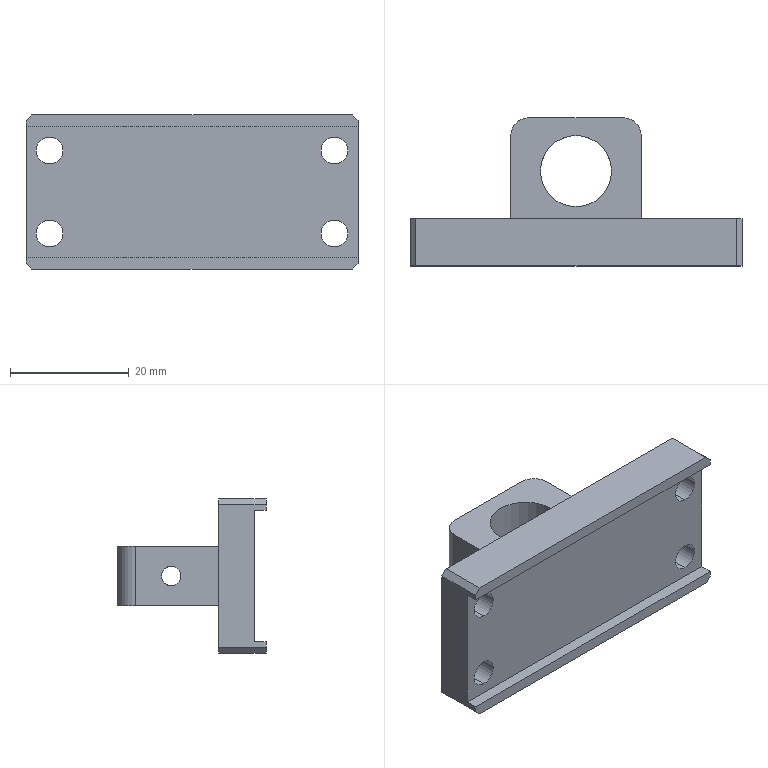Part | SolidWorks | features ICE 5, Fillet 2, HoleWzd 2, Chamfer 1, Extrusion 1 | 1 solid | 35 faces | box 56 x 25 x 26 mm | volume 11259 mm3 | plane 19 | cylinder 16 | commonest cylinder face diameters 4.5 x8 3.3 x4 6 x2 12 x2
STEP:
#1=CARTESIAN_POINT('',(-11.,16.,1.65));
#2=VERTEX_POINT('',#1);
#3=CARTESIAN_POINT('',(-11.,16.,-1.65));
#4=VERTEX_POINT('',#3);
#5=CARTESIAN_POINT('',(-11.,16.,0.));
#6=DIRECTION('',(1.,0.,0.));
#7=DIRECTION('',(0.,0.,-1.));
#8=AXIS2_PLACEMENT_3D('',#5,#6,#7);
#9=CIRCLE('',#8,1.65);
#10=EDGE_CURVE('',#2,#4,#9,.T.);
#11=ORIENTED_EDGE('',*,*,#10,.F.);
#12=CARTESIAN_POINT('',(-6.,16.,1.65));
#13=VERTEX_POINT('',#12);
#14=CARTESIAN_POINT('',(11.,16.,1.65));
#15=DIRECTION('',(1.,0.,0.));
#16=VECTOR('',#15,1000.);
#17=LINE('',#14,#16);
#18=EDGE_CURVE('',#2,#13,#17,.T.);
#19=ORIENTED_EDGE('',*,*,#18,.T.);
#20=CARTESIAN_POINT('',(-6.,16.,-1.65));
#21=VERTEX_POINT('',#20);
#22=CARTESIAN_POINT('',(-6.,16.,-1.65));
#23=CARTESIAN_POINT('',(-6.,15.784,-1.65));
#24=CARTESIAN_POINT('',(-5.988,15.566,-1.606));
#25=CARTESIAN_POINT('',(-5.956,15.268,-1.483));
#26=CARTESIAN_POINT('',(-5.943,15.171,-1.431));
#27=CARTESIAN_POINT('',(-5.915,14.992,-1.311));
#28=CARTESIAN_POINT('',(-5.901,14.91,-1.243));
#29=CARTESIAN_POINT('',(-5.87,14.757,-1.091));
#30=CARTESIAN_POINT('',(-5.855,14.688,-1.007));
#31=CARTESIAN_POINT('',(-5.827,14.569,-0.8288));
#32=CARTESIAN_POINT('',(-5.814,14.518,-0.7342));
#33=CARTESIAN_POINT('',(-5.792,14.435,-0.5332));
#34=CARTESIAN_POINT('',(-5.784,14.403,-0.4297));
#35=CARTESIAN_POINT('',(-5.772,14.361,-0.2184));
#36=CARTESIAN_POINT('',(-5.769,14.35,-0.1091));
#37=CARTESIAN_POINT('',(-5.769,14.35,0.1085));
#38=CARTESIAN_POINT('',(-5.772,14.361,0.2159));
#39=CARTESIAN_POINT('',(-5.784,14.403,0.4281));
#40=CARTESIAN_POINT('',(-5.792,14.435,0.5334));
#41=CARTESIAN_POINT('',(-5.825,14.559,0.8317));
#42=CARTESIAN_POINT('',(-5.855,14.681,1.015));
#43=CARTESIAN_POINT('',(-5.915,14.984,1.318));
#44=CARTESIAN_POINT('',(-5.945,15.167,1.44));
#45=CARTESIAN_POINT('',(-5.977,15.465,1.565));
#46=CARTESIAN_POINT('',(-5.986,15.57,1.597));
#47=CARTESIAN_POINT('',(-5.997,15.783,1.639));
#48=CARTESIAN_POINT('',(-6.,15.89,1.65));
#49=CARTESIAN_POINT('',(-6.,16.,1.65));
#50=B_SPLINE_CURVE_WITH_KNOTS('',3,(#22,#23,#24,#25,#26,#27,#28,#29,#30,#31,#32,#33,#34,#35,#36,#37,#38,#39,#40,#41,#42,#43,#44,#45,#46,#47,#48,#49),.UNSPECIFIED.,.F.,.F.,(4,2,2,2,2,2,2,2,2,2,2,2,2,4),(0.005184,0.005832,0.006155,0.006479,0.006803,0.007127,0.007451,0.007775,0.008099,0.008423,0.00907,0.009718,0.01004,0.01037),.UNSPECIFIED.);
#51=EDGE_CURVE('',#21,#13,#50,.T.);
#52=ORIENTED_EDGE('',*,*,#51,.F.);
#53=CARTESIAN_POINT('',(11.,16.,-1.65));
#54=DIRECTION('',(1.,0.,0.));
#55=VECTOR('',#54,1000.);
#56=LINE('',#53,#55);
#57=EDGE_CURVE('',#4,#21,#56,.T.);
#58=ORIENTED_EDGE('',*,*,#57,.F.);
#59=EDGE_LOOP('',(#11,#19,#52,#58));
#60=FACE_OUTER_BOUND('',#59,.T.);
#61=CARTESIAN_POINT('',(11.,16.,0.));
#62=DIRECTION('',(1.,0.,0.));
#63=DIRECTION('',(0.,0.,-1.));
#64=AXIS2_PLACEMENT_3D('',#61,#62,#63);
#65=CYLINDRICAL_SURFACE('',#64,1.65);
#66=ADVANCED_FACE('',(#60),#65,.F.);
#67=CARTESIAN_POINT('',(6.,16.,1.65));
#68=VERTEX_POINT('',#67);
#69=CARTESIAN_POINT('',(6.,16.,-1.65));
#70=VERTEX_POINT('',#69);
#71=CARTESIAN_POINT('',(6.,16.,1.65));
#72=CARTESIAN_POINT('',(6.,15.784,1.65));
#73=CARTESIAN_POINT('',(5.988,15.566,1.606));
#74=CARTESIAN_POINT('',(5.956,15.268,1.483));
#75=CARTESIAN_POINT('',(5.943,15.171,1.431));
#76=CARTESIAN_POINT('',(5.915,14.992,1.311));
#77=CARTESIAN_POINT('',(5.901,14.91,1.243));
#78=CARTESIAN_POINT('',(5.87,14.757,1.091));
#79=CARTESIAN_POINT('',(5.855,14.688,1.007));
#80=CARTESIAN_POINT('',(5.827,14.569,0.8288));
#81=CARTESIAN_POINT('',(5.814,14.518,0.7342));
#82=CARTESIAN_POINT('',(5.792,14.435,0.5332));
#83=CARTESIAN_POINT('',(5.784,14.403,0.4297));
#84=CARTESIAN_POINT('',(5.772,14.361,0.2184));
#85=CARTESIAN_POINT('',(5.769,14.35,0.1091));
#86=CARTESIAN_POINT('',(5.769,14.35,-0.1085));
#87=CARTESIAN_POINT('',(5.772,14.361,-0.2159));
#88=CARTESIAN_POINT('',(5.784,14.403,-0.4281));
#89=CARTESIAN_POINT('',(5.792,14.435,-0.5334));
#90=CARTESIAN_POINT('',(5.825,14.559,-0.8317));
#91=CARTESIAN_POINT('',(5.855,14.681,-1.015));
#92=CARTESIAN_POINT('',(5.915,14.984,-1.318));
#93=CARTESIAN_POINT('',(5.945,15.167,-1.44));
#94=CARTESIAN_POINT('',(5.977,15.465,-1.565));
#95=CARTESIAN_POINT('',(5.986,15.57,-1.597));
#96=CARTESIAN_POINT('',(5.997,15.783,-1.639));
#97=CARTESIAN_POINT('',(6.,15.89,-1.65));
#98=CARTESIAN_POINT('',(6.,16.,-1.65));
#99=B_SPLINE_CURVE_WITH_KNOTS('',3,(#71,#72,#73,#74,#75,#76,#77,#78,#79,#80,#81,#82,#83,#84,#85,#86,#87,#88,#89,#90,#91,#92,#93,#94,#95,#96,#97,#98),.UNSPECIFIED.,.F.,.F.,(4,2,2,2,2,2,2,2,2,2,2,2,2,4),(0.005184,0.005832,0.006155,0.006479,0.006803,0.007127,0.007451,0.007775,0.008099,0.008423,0.00907,0.009718,0.01004,0.01037),.UNSPECIFIED.);
#100=EDGE_CURVE('',#68,#70,#99,.T.);
#101=ORIENTED_EDGE('',*,*,#100,.F.);
#102=CARTESIAN_POINT('',(11.,16.,1.65));
#103=VERTEX_POINT('',#102);
#104=CARTESIAN_POINT('',(11.,16.,1.65));
#105=DIRECTION('',(1.,0.,0.));
#106=VECTOR('',#105,1000.);
#107=LINE('',#104,#106);
#108=EDGE_CURVE('',#68,#103,#107,.T.);
#109=ORIENTED_EDGE('',*,*,#108,.T.);
#110=CARTESIAN_POINT('',(11.,16.,-1.65));
#111=VERTEX_POINT('',#110);
#112=CARTESIAN_POINT('',(11.,16.,0.));
#113=DIRECTION('',(1.,0.,0.));
#114=DIRECTION('',(0.,0.,-1.));
#115=AXIS2_PLACEMENT_3D('',#112,#113,#114);
#116=CIRCLE('',#115,1.65);
#117=EDGE_CURVE('',#103,#111,#116,.T.);
#118=ORIENTED_EDGE('',*,*,#117,.T.);
#119=CARTESIAN_POINT('',(11.,16.,-1.65));
#120=DIRECTION('',(1.,0.,0.));
#121=VECTOR('',#120,1000.);
#122=LINE('',#119,#121);
#123=EDGE_CURVE('',#70,#111,#122,.T.);
#124=ORIENTED_EDGE('',*,*,#123,.F.);
#125=EDGE_LOOP('',(#101,#109,#118,#124));
#126=FACE_OUTER_BOUND('',#125,.T.);
#127=CARTESIAN_POINT('',(11.,16.,0.));
#128=DIRECTION('',(1.,0.,0.));
#129=DIRECTION('',(0.,0.,-1.));
#130=AXIS2_PLACEMENT_3D('',#127,#128,#129);
#131=CYLINDRICAL_SURFACE('',#130,1.65);
#132=ADVANCED_FACE('',(#126),#131,.F.);
#133=CARTESIAN_POINT('',(-24.,2.,-4.75));
#134=VERTEX_POINT('',#133);
#135=CARTESIAN_POINT('',(-24.,2.,-9.25));
#136=VERTEX_POINT('',#135);
#137=CARTESIAN_POINT('',(-24.,2.,-7.));
#138=DIRECTION('',(0.,-1.,0.));
#139=DIRECTION('',(0.,0.,-1.));
#140=AXIS2_PLACEMENT_3D('',#137,#138,#139);
#141=CIRCLE('',#140,2.25);
#142=EDGE_CURVE('',#134,#136,#141,.T.);
#143=ORIENTED_EDGE('',*,*,#142,.T.);
#144=CARTESIAN_POINT('',(-24.,8.,-9.25));
#145=VERTEX_POINT('',#144);
#146=CARTESIAN_POINT('',(-24.,8.,-9.25));
#147=DIRECTION('',(0.,1.,0.));
#148=VECTOR('',#147,1000.);
#149=LINE('',#146,#148);
#150=EDGE_CURVE('',#136,#145,#149,.T.);
#151=ORIENTED_EDGE('',*,*,#150,.T.);
#152=CARTESIAN_POINT('',(-24.,8.,-4.75));
#153=VERTEX_POINT('',#152);
#154=CARTESIAN_POINT('',(-24.,8.,-7.));
#155=DIRECTION('',(0.,1.,0.));
#156=DIRECTION('',(0.,0.,1.));
#157=AXIS2_PLACEMENT_3D('',#154,#155,#156);
#158=CIRCLE('',#157,2.25);
#159=EDGE_CURVE('',#145,#153,#158,.T.);
#160=ORIENTED_EDGE('',*,*,#159,.T.);
#161=CARTESIAN_POINT('',(-24.,8.,-4.75));
#162=DIRECTION('',(0.,1.,0.));
#163=VECTOR('',#162,1000.);
#164=LINE('',#161,#163);
#165=EDGE_CURVE('',#134,#153,#164,.T.);
#166=ORIENTED_EDGE('',*,*,#165,.F.);
#167=EDGE_LOOP('',(#143,#151,#160,#166));
#168=FACE_OUTER_BOUND('',#167,.T.);
#169=CARTESIAN_POINT('',(-24.,8.,-7.));
#170=DIRECTION('',(0.,1.,0.));
#171=DIRECTION('',(0.,0.,1.));
#172=AXIS2_PLACEMENT_3D('',#169,#170,#171);
#173=CYLINDRICAL_SURFACE('',#172,2.25);
#174=ADVANCED_FACE('',(#168),#173,.F.);
#175=CARTESIAN_POINT('',(-24.,2.,9.25));
#176=VERTEX_POINT('',#175);
#177=CARTESIAN_POINT('',(-24.,2.,4.75));
#178=VERTEX_POINT('',#177);
#179=CARTESIAN_POINT('',(-24.,2.,7.));
#180=DIRECTION('',(0.,-1.,0.));
#181=DIRECTION('',(0.,0.,-1.));
#182=AXIS2_PLACEMENT_3D('',#179,#180,#181);
#183=CIRCLE('',#182,2.25);
#184=EDGE_CURVE('',#176,#178,#183,.T.);
#185=ORIENTED_EDGE('',*,*,#184,.T.);
#186=CARTESIAN_POINT('',(-24.,8.,4.75));
#187=VERTEX_POINT('',#186);
#188=CARTESIAN_POINT('',(-24.,8.,4.75));
#189=DIRECTION('',(0.,1.,0.));
#190=VECTOR('',#189,1000.);
#191=LINE('',#188,#190);
#192=EDGE_CURVE('',#178,#187,#191,.T.);
#193=ORIENTED_EDGE('',*,*,#192,.T.);
#194=CARTESIAN_POINT('',(-24.,8.,9.25));
#195=VERTEX_POINT('',#194);
#196=CARTESIAN_POINT('',(-24.,8.,7.));
#197=DIRECTION('',(0.,1.,0.));
#198=DIRECTION('',(0.,0.,1.));
#199=AXIS2_PLACEMENT_3D('',#196,#197,#198);
#200=CIRCLE('',#199,2.25);
#201=EDGE_CURVE('',#187,#195,#200,.T.);
#202=ORIENTED_EDGE('',*,*,#201,.T.);
#203=CARTESIAN_POINT('',(-24.,8.,9.25));
#204=DIRECTION('',(0.,1.,0.));
#205=VECTOR('',#204,1000.);
#206=LINE('',#203,#205);
#207=EDGE_CURVE('',#176,#195,#206,.T.);
#208=ORIENTED_EDGE('',*,*,#207,.F.);
#209=EDGE_LOOP('',(#185,#193,#202,#208));
#210=FACE_OUTER_BOUND('',#209,.T.);
#211=CARTESIAN_POINT('',(-24.,8.,7.));
#212=DIRECTION('',(0.,1.,0.));
#213=DIRECTION('',(0.,0.,1.));
#214=AXIS2_PLACEMENT_3D('',#211,#212,#213);
#215=CYLINDRICAL_SURFACE('',#214,2.25);
#216=ADVANCED_FACE('',(#210),#215,.F.);
#217=CARTESIAN_POINT('',(24.,2.,-4.75));
#218=VERTEX_POINT('',#217);
#219=CARTESIAN_POINT('',(24.,2.,-9.25));
#220=VERTEX_POINT('',#219);
#221=CARTESIAN_POINT('',(24.,2.,-7.));
#222=DIRECTION('',(0.,-1.,0.));
#223=DIRECTION('',(0.,0.,-1.));
#224=AXIS2_PLACEMENT_3D('',#221,#222,#223);
#225=CIRCLE('',#224,2.25);
#226=EDGE_CURVE('',#218,#220,#225,.T.);
#227=ORIENTED_EDGE('',*,*,#226,.T.);
#228=CARTESIAN_POINT('',(24.,8.,-9.25));
#229=VERTEX_POINT('',#228);
#230=CARTESIAN_POINT('',(24.,8.,-9.25));
#231=DIRECTION('',(0.,1.,0.));
#232=VECTOR('',#231,1000.);
#233=LINE('',#230,#232);
#234=EDGE_CURVE('',#220,#229,#233,.T.);
#235=ORIENTED_EDGE('',*,*,#234,.T.);
#236=CARTESIAN_POINT('',(24.,8.,-4.75));
#237=VERTEX_POINT('',#236);
#238=CARTESIAN_POINT('',(24.,8.,-7.));
#239=DIRECTION('',(0.,1.,0.));
#240=DIRECTION('',(0.,0.,1.));
#241=AXIS2_PLACEMENT_3D('',#238,#239,#240);
#242=CIRCLE('',#241,2.25);
#243=EDGE_CURVE('',#229,#237,#242,.T.);
#244=ORIENTED_EDGE('',*,*,#243,.T.);
#245=CARTESIAN_POINT('',(24.,8.,-4.75));
#246=DIRECTION('',(0.,1.,0.));
#247=VECTOR('',#246,1000.);
#248=LINE('',#245,#247);
#249=EDGE_CURVE('',#218,#237,#248,.T.);
#250=ORIENTED_EDGE('',*,*,#249,.F.);
#251=EDGE_LOOP('',(#227,#235,#244,#250));
#252=FACE_OUTER_BOUND('',#251,.T.);
#253=CARTESIAN_POINT('',(24.,8.,-7.));
#254=DIRECTION('',(0.,1.,0.));
#255=DIRECTION('',(0.,0.,1.));
#256=AXIS2_PLACEMENT_3D('',#253,#254,#255);
#257=CYLINDRICAL_SURFACE('',#256,2.25);
#258=ADVANCED_FACE('',(#252),#257,.F.);
#259=CARTESIAN_POINT('',(24.,2.,9.25));
#260=VERTEX_POINT('',#259);
#261=CARTESIAN_POINT('',(24.,2.,4.75));
#262=VERTEX_POINT('',#261);
#263=CARTESIAN_POINT('',(24.,2.,7.));
#264=DIRECTION('',(0.,-1.,0.));
#265=DIRECTION('',(0.,0.,-1.));
#266=AXIS2_PLACEMENT_3D('',#263,#264,#265);
#267=CIRCLE('',#266,2.25);
#268=EDGE_CURVE('',#260,#262,#267,.T.);
#269=ORIENTED_EDGE('',*,*,#268,.T.);
#270=CARTESIAN_POINT('',(24.,8.,4.75));
#271=VERTEX_POINT('',#270);
#272=CARTESIAN_POINT('',(24.,8.,4.75));
#273=DIRECTION('',(0.,1.,0.));
#274=VECTOR('',#273,1000.);
#275=LINE('',#272,#274);
#276=EDGE_CURVE('',#262,#271,#275,.T.);
#277=ORIENTED_EDGE('',*,*,#276,.T.);
#278=CARTESIAN_POINT('',(24.,8.,9.25));
#279=VERTEX_POINT('',#278);
#280=CARTESIAN_POINT('',(24.,8.,7.));
#281=DIRECTION('',(0.,1.,0.));
#282=DIRECTION('',(0.,0.,1.));
#283=AXIS2_PLACEMENT_3D('',#280,#281,#282);
#284=CIRCLE('',#283,2.25);
#285=EDGE_CURVE('',#271,#279,#284,.T.);
#286=ORIENTED_EDGE('',*,*,#285,.T.);
#287=CARTESIAN_POINT('',(24.,8.,9.25));
#288=DIRECTION('',(0.,1.,0.));
#289=VECTOR('',#288,1000.);
#290=LINE('',#287,#289);
#291=EDGE_CURVE('',#260,#279,#290,.T.);
#292=ORIENTED_EDGE('',*,*,#291,.F.);
#293=EDGE_LOOP('',(#269,#277,#286,#292));
#294=FACE_OUTER_BOUND('',#293,.T.);
#295=CARTESIAN_POINT('',(24.,8.,7.));
#296=DIRECTION('',(0.,1.,0.));
#297=DIRECTION('',(0.,0.,1.));
#298=AXIS2_PLACEMENT_3D('',#295,#296,#297);
#299=CYLINDRICAL_SURFACE('',#298,2.25);
#300=ADVANCED_FACE('',(#294),#299,.F.);
#301=CARTESIAN_POINT('',(6.,16.,5.));
#302=VERTEX_POINT('',#301);
#303=CARTESIAN_POINT('',(-6.,16.,5.));
#304=VERTEX_POINT('',#303);
#305=CARTESIAN_POINT('',(0.,16.,5.));
#306=DIRECTION('',(0.,0.,-1.));
#307=DIRECTION('',(-1.,0.,0.));
#308=AXIS2_PLACEMENT_3D('',#305,#306,#307);
#309=CIRCLE('',#308,6.);
#310=EDGE_CURVE('',#302,#304,#309,.T.);
#311=ORIENTED_EDGE('',*,*,#310,.F.);
#312=CARTESIAN_POINT('',(6.,16.,13.));
#313=DIRECTION('',(0.,0.,-1.));
#314=VECTOR('',#313,1000.);
#315=LINE('',#312,#314);
#316=EDGE_CURVE('',#302,#68,#315,.T.);
#317=ORIENTED_EDGE('',*,*,#316,.T.);
#318=ORIENTED_EDGE('',*,*,#100,.T.);
#319=CARTESIAN_POINT('',(6.,16.,-5.));
#320=VERTEX_POINT('',#319);
#321=CARTESIAN_POINT('',(6.,16.,13.));
#322=DIRECTION('',(0.,0.,-1.));
#323=VECTOR('',#322,1000.);
#324=LINE('',#321,#323);
#325=EDGE_CURVE('',#70,#320,#324,.T.);
#326=ORIENTED_EDGE('',*,*,#325,.T.);
#327=CARTESIAN_POINT('',(-6.,16.,-5.));
#328=VERTEX_POINT('',#327);
#329=CARTESIAN_POINT('',(0.,16.,-5.));
#330=DIRECTION('',(0.,0.,1.));
#331=DIRECTION('',(1.,0.,0.));
#332=AXIS2_PLACEMENT_3D('',#329,#330,#331);
#333=CIRCLE('',#332,6.);
#334=EDGE_CURVE('',#328,#320,#333,.T.);
#335=ORIENTED_EDGE('',*,*,#334,.F.);
#336=CARTESIAN_POINT('',(-6.,16.,13.));
#337=DIRECTION('',(0.,0.,-1.));
#338=VECTOR('',#337,1000.);
#339=LINE('',#336,#338);
#340=EDGE_CURVE('',#21,#328,#339,.T.);
#341=ORIENTED_EDGE('',*,*,#340,.F.);
#342=ORIENTED_EDGE('',*,*,#51,.T.);
#343=CARTESIAN_POINT('',(-6.,16.,13.));
#344=DIRECTION('',(0.,0.,-1.));
#345=VECTOR('',#344,1000.);
#346=LINE('',#343,#345);
#347=EDGE_CURVE('',#304,#13,#346,.T.);
#348=ORIENTED_EDGE('',*,*,#347,.F.);
#349=EDGE_LOOP('',(#311,#317,#318,#326,#335,#341,#342,#348));
#350=FACE_OUTER_BOUND('',#349,.T.);
#351=CARTESIAN_POINT('',(0.,16.,13.));
#352=DIRECTION('',(0.,0.,-1.));
#353=DIRECTION('',(-1.,0.,0.));
#354=AXIS2_PLACEMENT_3D('',#351,#352,#353);
#355=CYLINDRICAL_SURFACE('',#354,6.);
#356=ADVANCED_FACE('',(#350),#355,.F.);
#357=CARTESIAN_POINT('',(-24.,8.,-7.));
#358=DIRECTION('',(0.,1.,0.));
#359=DIRECTION('',(0.,0.,1.));
#360=AXIS2_PLACEMENT_3D('',#357,#358,#359);
#361=CIRCLE('',#360,2.25);
#362=EDGE_CURVE('',#153,#145,#361,.T.);
#363=ORIENTED_EDGE('',*,*,#362,.F.);
#364=ORIENTED_EDGE('',*,*,#159,.F.);
#365=EDGE_LOOP('',(#363,#364));
#366=FACE_BOUND('',#365,.T.);
#367=CARTESIAN_POINT('',(-24.,8.,7.));
#368=DIRECTION('',(0.,1.,0.));
#369=DIRECTION('',(0.,0.,1.));
#370=AXIS2_PLACEMENT_3D('',#367,#368,#369);
#371=CIRCLE('',#370,2.25);
#372=EDGE_CURVE('',#195,#187,#371,.T.);
#373=ORIENTED_EDGE('',*,*,#372,.F.);
#374=ORIENTED_EDGE('',*,*,#201,.F.);
#375=EDGE_LOOP('',(#373,#374));
#376=FACE_BOUND('',#375,.T.);
#377=CARTESIAN_POINT('',(24.,8.,-7.));
#378=DIRECTION('',(0.,1.,0.));
#379=DIRECTION('',(0.,0.,1.));
#380=AXIS2_PLACEMENT_3D('',#377,#378,#379);
#381=CIRCLE('',#380,2.25);
#382=EDGE_CURVE('',#237,#229,#381,.T.);
#383=ORIENTED_EDGE('',*,*,#382,.F.);
#384=ORIENTED_EDGE('',*,*,#243,.F.);
#385=EDGE_LOOP('',(#383,#384));
#386=FACE_BOUND('',#385,.T.);
#387=CARTESIAN_POINT('',(24.,8.,7.));
#388=DIRECTION('',(0.,1.,0.));
#389=DIRECTION('',(0.,0.,1.));
#390=AXIS2_PLACEMENT_3D('',#387,#388,#389);
#391=CIRCLE('',#390,2.25);
#392=EDGE_CURVE('',#279,#271,#391,.T.);
#393=ORIENTED_EDGE('',*,*,#392,.F.);
#394=ORIENTED_EDGE('',*,*,#285,.F.);
#395=EDGE_LOOP('',(#393,#394));
#396=FACE_BOUND('',#395,.T.);
#397=CARTESIAN_POINT('',(27.,8.,-13.));
#398=VERTEX_POINT('',#397);
#399=CARTESIAN_POINT('',(-27.,8.,-13.));
#400=VERTEX_POINT('',#399);
#401=CARTESIAN_POINT('',(-28.,8.,-13.));
#402=DIRECTION('',(-1.,0.,0.));
#403=VECTOR('',#402,1000.);
#404=LINE('',#401,#403);
#405=EDGE_CURVE('',#398,#400,#404,.T.);
#406=ORIENTED_EDGE('',*,*,#405,.T.);
#407=CARTESIAN_POINT('',(-28.,8.,-12.));
#408=VERTEX_POINT('',#407);
#409=CARTESIAN_POINT('',(-20.,8.,-20.));
#410=DIRECTION('',(-0.7071,0.,0.7071));
#411=VECTOR('',#410,1000.);
#412=LINE('',#409,#411);
#413=EDGE_CURVE('',#400,#408,#412,.T.);
#414=ORIENTED_EDGE('',*,*,#413,.T.);
#415=CARTESIAN_POINT('',(-28.,8.,12.));
#416=VERTEX_POINT('',#415);
#417=CARTESIAN_POINT('',(-28.,8.,-13.));
#418=DIRECTION('',(0.,0.,1.));
#419=VECTOR('',#418,1000.);
#420=LINE('',#417,#419);
#421=EDGE_CURVE('',#408,#416,#420,.T.);
#422=ORIENTED_EDGE('',*,*,#421,.T.);
#423=CARTESIAN_POINT('',(-27.,8.,13.));
#424=VERTEX_POINT('',#423);
#425=CARTESIAN_POINT('',(-20.,8.,20.));
#426=DIRECTION('',(0.7071,0.,0.7071));
#427=VECTOR('',#426,1000.);
#428=LINE('',#425,#427);
#429=EDGE_CURVE('',#416,#424,#428,.T.);
#430=ORIENTED_EDGE('',*,*,#429,.T.);
#431=CARTESIAN_POINT('',(27.,8.,13.));
#432=VERTEX_POINT('',#431);
#433=CARTESIAN_POINT('',(-28.,8.,13.));
#434=DIRECTION('',(1.,0.,0.));
#435=VECTOR('',#434,1000.);
#436=LINE('',#433,#435);
#437=EDGE_CURVE('',#424,#432,#436,.T.);
#438=ORIENTED_EDGE('',*,*,#437,.T.);
#439=CARTESIAN_POINT('',(28.,8.,12.));
#440=VERTEX_POINT('',#439);
#441=CARTESIAN_POINT('',(20.,8.,20.));
#442=DIRECTION('',(0.7071,0.,-0.7071));
#443=VECTOR('',#442,1000.);
#444=LINE('',#441,#443);
#445=EDGE_CURVE('',#432,#440,#444,.T.);
#446=ORIENTED_EDGE('',*,*,#445,.T.);
#447=CARTESIAN_POINT('',(28.,8.,-12.));
#448=VERTEX_POINT('',#447);
#449=CARTESIAN_POINT('',(28.,8.,-13.));
#450=DIRECTION('',(0.,0.,-1.));
#451=VECTOR('',#450,1000.);
#452=LINE('',#449,#451);
#453=EDGE_CURVE('',#440,#448,#452,.T.);
#454=ORIENTED_EDGE('',*,*,#453,.T.);
#455=CARTESIAN_POINT('',(20.,8.,-20.));
#456=DIRECTION('',(-0.7071,0.,-0.7071));
#457=VECTOR('',#456,1000.);
#458=LINE('',#455,#457);
#459=EDGE_CURVE('',#448,#398,#458,.T.);
#460=ORIENTED_EDGE('',*,*,#459,.T.);
#461=EDGE_LOOP('',(#406,#414,#422,#430,#438,#446,#454,#460));
#462=FACE_OUTER_BOUND('',#461,.T.);
#463=CARTESIAN_POINT('',(11.,8.,-5.));
#464=VERTEX_POINT('',#463);
#465=CARTESIAN_POINT('',(-11.,8.,-5.));
#466=VERTEX_POINT('',#465);
#467=CARTESIAN_POINT('',(-11.,8.,-5.));
#468=DIRECTION('',(-1.,0.,0.));
#469=VECTOR('',#468,1000.);
#470=LINE('',#467,#469);
#471=EDGE_CURVE('',#464,#466,#470,.T.);
#472=ORIENTED_EDGE('',*,*,#471,.F.);
#473=CARTESIAN_POINT('',(11.,8.,5.));
#474=VERTEX_POINT('',#473);
#475=CARTESIAN_POINT('',(11.,8.,-5.));
#476=DIRECTION('',(0.,0.,-1.));
#477=VECTOR('',#476,1000.);
#478=LINE('',#475,#477);
#479=EDGE_CURVE('',#474,#464,#478,.T.);
#480=ORIENTED_EDGE('',*,*,#479,.F.);
#481=CARTESIAN_POINT('',(-11.,8.,5.));
#482=VERTEX_POINT('',#481);
#483=CARTESIAN_POINT('',(-11.,8.,5.));
#484=DIRECTION('',(1.,0.,0.));
#485=VECTOR('',#484,1000.);
#486=LINE('',#483,#485);
#487=EDGE_CURVE('',#482,#474,#486,.T.);
#488=ORIENTED_EDGE('',*,*,#487,.F.);
#489=CARTESIAN_POINT('',(-11.,8.,-5.));
#490=DIRECTION('',(0.,0.,1.));
#491=VECTOR('',#490,1000.);
#492=LINE('',#489,#491);
#493=EDGE_CURVE('',#466,#482,#492,.T.);
#494=ORIENTED_EDGE('',*,*,#493,.F.);
#495=EDGE_LOOP('',(#472,#480,#488,#494));
#496=FACE_BOUND('',#495,.T.);
#497=CARTESIAN_POINT('',(0.,8.,0.));
#498=DIRECTION('',(0.,1.,0.));
#499=DIRECTION('',(0.,0.,1.));
#500=AXIS2_PLACEMENT_3D('',#497,#498,#499);
#501=PLANE('',#500);
#502=ADVANCED_FACE('',(#366,#376,#386,#396,#462,#496),#501,.T.);
#503=CARTESIAN_POINT('',(-28.,0.,-12.));
#504=VERTEX_POINT('',#503);
#505=CARTESIAN_POINT('',(-28.,0.,-11.05));
#506=VERTEX_POINT('',#505);
#507=CARTESIAN_POINT('',(-28.,0.,-13.));
#508=DIRECTION('',(0.,0.,1.));
#509=VECTOR('',#508,1000.);
#510=LINE('',#507,#509);
#511=EDGE_CURVE('',#504,#506,#510,.T.);
#512=ORIENTED_EDGE('',*,*,#511,.F.);
#513=CARTESIAN_POINT('',(-27.,0.,-13.));
#514=VERTEX_POINT('',#513);
#515=CARTESIAN_POINT('',(-28.,0.,-12.));
#516=DIRECTION('',(0.7071,0.,-0.7071));
#517=VECTOR('',#516,1000.);
#518=LINE('',#515,#517);
#519=EDGE_CURVE('',#504,#514,#518,.T.);
#520=ORIENTED_EDGE('',*,*,#519,.T.);
#521=CARTESIAN_POINT('',(27.,0.,-13.));
#522=VERTEX_POINT('',#521);
#523=CARTESIAN_POINT('',(-28.,0.,-13.));
#524=DIRECTION('',(-1.,0.,0.));
#525=VECTOR('',#524,1000.);
#526=LINE('',#523,#525);
#527=EDGE_CURVE('',#522,#514,#526,.T.);
#528=ORIENTED_EDGE('',*,*,#527,.F.);
#529=CARTESIAN_POINT('',(28.,0.,-12.));
#530=VERTEX_POINT('',#529);
#531=CARTESIAN_POINT('',(27.,0.,-13.));
#532=DIRECTION('',(0.7071,0.,0.7071));
#533=VECTOR('',#532,1000.);
#534=LINE('',#531,#533);
#535=EDGE_CURVE('',#522,#530,#534,.T.);
#536=ORIENTED_EDGE('',*,*,#535,.T.);
#537=CARTESIAN_POINT('',(28.,0.,-11.05));
#538=VERTEX_POINT('',#537);
#539=CARTESIAN_POINT('',(28.,0.,-13.));
#540=DIRECTION('',(0.,0.,-1.));
#541=VECTOR('',#540,1000.);
#542=LINE('',#539,#541);
#543=EDGE_CURVE('',#538,#530,#542,.T.);
#544=ORIENTED_EDGE('',*,*,#543,.F.);
#545=CARTESIAN_POINT('',(0.,0.,-11.05));
#546=DIRECTION('',(-1.,0.,0.));
#547=VECTOR('',#546,1000.);
#548=LINE('',#545,#547);
#549=EDGE_CURVE('',#538,#506,#548,.T.);
#550=ORIENTED_EDGE('',*,*,#549,.T.);
#551=EDGE_LOOP('',(#512,#520,#528,#536,#544,#550));
#552=FACE_OUTER_BOUND('',#551,.T.);
#553=CARTESIAN_POINT('',(0.,0.,0.));
#554=DIRECTION('',(0.,1.,0.));
#555=DIRECTION('',(0.,0.,1.));
#556=AXIS2_PLACEMENT_3D('',#553,#554,#555);
#557=PLANE('',#556);
#558=ADVANCED_FACE('',(#552),#557,.F.);
#559=ORIENTED_EDGE('',*,*,#453,.F.);
#560=CARTESIAN_POINT('',(28.,0.,12.));
#561=VERTEX_POINT('',#560);
#562=CARTESIAN_POINT('',(28.,8.,12.));
#563=DIRECTION('',(0.,-1.,0.));
#564=VECTOR('',#563,1000.);
#565=LINE('',#562,#564);
#566=EDGE_CURVE('',#440,#561,#565,.T.);
#567=ORIENTED_EDGE('',*,*,#566,.T.);
#568=CARTESIAN_POINT('',(28.,0.,11.05));
#569=VERTEX_POINT('',#568);
#570=CARTESIAN_POINT('',(28.,0.,-13.));
#571=DIRECTION('',(0.,0.,-1.));
#572=VECTOR('',#571,1000.);
#573=LINE('',#570,#572);
#574=EDGE_CURVE('',#561,#569,#573,.T.);
#575=ORIENTED_EDGE('',*,*,#574,.T.);
#576=CARTESIAN_POINT('',(28.,2.,11.05));
#577=VERTEX_POINT('',#576);
#578=CARTESIAN_POINT('',(28.,8.,11.05));
#579=DIRECTION('',(0.,1.,0.));
#580=VECTOR('',#579,1000.);
#581=LINE('',#578,#580);
#582=EDGE_CURVE('',#569,#577,#581,.T.);
#583=ORIENTED_EDGE('',*,*,#582,.T.);
#584=CARTESIAN_POINT('',(28.,2.,-11.05));
#585=VERTEX_POINT('',#584);
#586=CARTESIAN_POINT('',(28.,2.,-13.));
#587=DIRECTION('',(0.,0.,1.));
#588=VECTOR('',#587,1000.);
#589=LINE('',#586,#588);
#590=EDGE_CURVE('',#585,#577,#589,.T.);
#591=ORIENTED_EDGE('',*,*,#590,.F.);
#592=CARTESIAN_POINT('',(28.,8.,-11.05));
#593=DIRECTION('',(0.,-1.,0.));
#594=VECTOR('',#593,1000.);
#595=LINE('',#592,#594);
#596=EDGE_CURVE('',#585,#538,#595,.T.);
#597=ORIENTED_EDGE('',*,*,#596,.T.);
#598=ORIENTED_EDGE('',*,*,#543,.T.);
#599=CARTESIAN_POINT('',(28.,8.,-12.));
#600=DIRECTION('',(0.,1.,0.));
#601=VECTOR('',#600,1000.);
#602=LINE('',#599,#601);
#603=EDGE_CURVE('',#530,#448,#602,.T.);
#604=ORIENTED_EDGE('',*,*,#603,.T.);
#605=EDGE_LOOP('',(#559,#567,#575,#583,#591,#597,#598,#604));
#606=FACE_OUTER_BOUND('',#605,.T.);
#607=CARTESIAN_POINT('',(28.,8.,-13.));
#608=DIRECTION('',(-1.,0.,0.));
#609=DIRECTION('',(0.,0.,1.));
#610=AXIS2_PLACEMENT_3D('',#607,#608,#609);
#611=PLANE('',#610);
#612=ADVANCED_FACE('',(#606),#611,.F.);
#613=ORIENTED_EDGE('',*,*,#527,.T.);
#614=CARTESIAN_POINT('',(-27.,8.,-13.));
#615=DIRECTION('',(0.,1.,0.));
#616=VECTOR('',#615,1000.);
#617=LINE('',#614,#616);
#618=EDGE_CURVE('',#514,#400,#617,.T.);
#619=ORIENTED_EDGE('',*,*,#618,.T.);
#620=ORIENTED_EDGE('',*,*,#405,.F.);
#621=CARTESIAN_POINT('',(27.,8.,-13.));
#622=DIRECTION('',(0.,-1.,0.));
#623=VECTOR('',#622,1000.);
#624=LINE('',#621,#623);
#625=EDGE_CURVE('',#398,#522,#624,.T.);
#626=ORIENTED_EDGE('',*,*,#625,.T.);
#627=EDGE_LOOP('',(#613,#619,#620,#626));
#628=FACE_OUTER_BOUND('',#627,.T.);
#629=CARTESIAN_POINT('',(-28.,8.,-13.));
#630=DIRECTION('',(0.,0.,1.));
#631=DIRECTION('',(1.,0.,0.));
#632=AXIS2_PLACEMENT_3D('',#629,#630,#631);
#633=PLANE('',#632);
#634=ADVANCED_FACE('',(#628),#633,.F.);
#635=ORIENTED_EDGE('',*,*,#421,.F.);
#636=CARTESIAN_POINT('',(-28.,8.,-12.));
#637=DIRECTION('',(0.,-1.,0.));
#638=VECTOR('',#637,1000.);
#639=LINE('',#636,#638);
#640=EDGE_CURVE('',#408,#504,#639,.T.);
#641=ORIENTED_EDGE('',*,*,#640,.T.);
#642=ORIENTED_EDGE('',*,*,#511,.T.);
#643=CARTESIAN_POINT('',(-28.,2.,-11.05));
#644=VERTEX_POINT('',#643);
#645=CARTESIAN_POINT('',(-28.,8.,-11.05));
#646=DIRECTION('',(0.,1.,0.));
#647=VECTOR('',#646,1000.);
#648=LINE('',#645,#647);
#649=EDGE_CURVE('',#506,#644,#648,.T.);
#650=ORIENTED_EDGE('',*,*,#649,.T.);
#651=CARTESIAN_POINT('',(-28.,2.,11.05));
#652=VERTEX_POINT('',#651);
#653=CARTESIAN_POINT('',(-28.,2.,-13.));
#654=DIRECTION('',(0.,0.,-1.));
#655=VECTOR('',#654,1000.);
#656=LINE('',#653,#655);
#657=EDGE_CURVE('',#652,#644,#656,.T.);
#658=ORIENTED_EDGE('',*,*,#657,.F.);
#659=CARTESIAN_POINT('',(-28.,0.,11.05));
#660=VERTEX_POINT('',#659);
#661=CARTESIAN_POINT('',(-28.,8.,11.05));
#662=DIRECTION('',(0.,-1.,0.));
#663=VECTOR('',#662,1000.);
#664=LINE('',#661,#663);
#665=EDGE_CURVE('',#652,#660,#664,.T.);
#666=ORIENTED_EDGE('',*,*,#665,.T.);
#667=CARTESIAN_POINT('',(-28.,0.,12.));
#668=VERTEX_POINT('',#667);
#669=CARTESIAN_POINT('',(-28.,0.,-13.));
#670=DIRECTION('',(0.,0.,1.));
#671=VECTOR('',#670,1000.);
#672=LINE('',#669,#671);
#673=EDGE_CURVE('',#660,#668,#672,.T.);
#674=ORIENTED_EDGE('',*,*,#673,.T.);
#675=CARTESIAN_POINT('',(-28.,8.,12.));
#676=DIRECTION('',(0.,1.,0.));
#677=VECTOR('',#676,1000.);
#678=LINE('',#675,#677);
#679=EDGE_CURVE('',#668,#416,#678,.T.);
#680=ORIENTED_EDGE('',*,*,#679,.T.);
#681=EDGE_LOOP('',(#635,#641,#642,#650,#658,#666,#674,#680));
#682=FACE_OUTER_BOUND('',#681,.T.);
#683=CARTESIAN_POINT('',(-28.,8.,-13.));
#684=DIRECTION('',(1.,0.,0.));
#685=DIRECTION('',(0.,0.,-1.));
#686=AXIS2_PLACEMENT_3D('',#683,#684,#685);
#687=PLANE('',#686);
#688=ADVANCED_FACE('',(#682),#687,.F.);
#689=ORIENTED_EDGE('',*,*,#437,.F.);
#690=CARTESIAN_POINT('',(-27.,0.,13.));
#691=VERTEX_POINT('',#690);
#692=CARTESIAN_POINT('',(-27.,8.,13.));
#693=DIRECTION('',(0.,-1.,0.));
#694=VECTOR('',#693,1000.);
#695=LINE('',#692,#694);
#696=EDGE_CURVE('',#424,#691,#695,.T.);
#697=ORIENTED_EDGE('',*,*,#696,.T.);
#698=CARTESIAN_POINT('',(27.,0.,13.));
#699=VERTEX_POINT('',#698);
#700=CARTESIAN_POINT('',(-28.,0.,13.));
#701=DIRECTION('',(1.,0.,0.));
#702=VECTOR('',#701,1000.);
#703=LINE('',#700,#702);
#704=EDGE_CURVE('',#691,#699,#703,.T.);
#705=ORIENTED_EDGE('',*,*,#704,.T.);
#706=CARTESIAN_POINT('',(27.,8.,13.));
#707=DIRECTION('',(0.,1.,0.));
#708=VECTOR('',#707,1000.);
#709=LINE('',#706,#708);
#710=EDGE_CURVE('',#699,#432,#709,.T.);
#711=ORIENTED_EDGE('',*,*,#710,.T.);
#712=EDGE_LOOP('',(#689,#697,#705,#711));
#713=FACE_OUTER_BOUND('',#712,.T.);
#714=CARTESIAN_POINT('',(-28.,8.,13.));
#715=DIRECTION('',(0.,0.,-1.));
#716=DIRECTION('',(-1.,0.,0.));
#717=AXIS2_PLACEMENT_3D('',#714,#715,#716);
#718=PLANE('',#717);
#719=ADVANCED_FACE('',(#713),#718,.F.);
#720=ORIENTED_EDGE('',*,*,#704,.F.);
#721=CARTESIAN_POINT('',(-27.,0.,13.));
#722=DIRECTION('',(-0.7071,0.,-0.7071));
#723=VECTOR('',#722,1000.);
#724=LINE('',#721,#723);
#725=EDGE_CURVE('',#691,#668,#724,.T.);
#726=ORIENTED_EDGE('',*,*,#725,.T.);
#727=ORIENTED_EDGE('',*,*,#673,.F.);
#728=CARTESIAN_POINT('',(0.,0.,11.05));
#729=DIRECTION('',(1.,0.,0.));
#730=VECTOR('',#729,1000.);
#731=LINE('',#728,#730);
#732=EDGE_CURVE('',#660,#569,#731,.T.);
#733=ORIENTED_EDGE('',*,*,#732,.T.);
#734=ORIENTED_EDGE('',*,*,#574,.F.);
#735=CARTESIAN_POINT('',(28.,0.,12.));
#736=DIRECTION('',(-0.7071,0.,0.7071));
#737=VECTOR('',#736,1000.);
#738=LINE('',#735,#737);
#739=EDGE_CURVE('',#561,#699,#738,.T.);
#740=ORIENTED_EDGE('',*,*,#739,.T.);
#741=EDGE_LOOP('',(#720,#726,#727,#733,#734,#740));
#742=FACE_OUTER_BOUND('',#741,.T.);
#743=CARTESIAN_POINT('',(0.,0.,0.));
#744=DIRECTION('',(0.,1.,0.));
#745=DIRECTION('',(0.,0.,1.));
#746=AXIS2_PLACEMENT_3D('',#743,#744,#745);
#747=PLANE('',#746);
#748=ADVANCED_FACE('',(#742),#747,.F.);
#749=ORIENTED_EDGE('',*,*,#142,.F.);
#750=CARTESIAN_POINT('',(-24.,2.,-7.));
#751=DIRECTION('',(0.,-1.,0.));
#752=DIRECTION('',(0.,0.,-1.));
#753=AXIS2_PLACEMENT_3D('',#750,#751,#752);
#754=CIRCLE('',#753,2.25);
#755=EDGE_CURVE('',#136,#134,#754,.T.);
#756=ORIENTED_EDGE('',*,*,#755,.F.);
#757=EDGE_LOOP('',(#749,#756));
#758=FACE_BOUND('',#757,.T.);
#759=ORIENTED_EDGE('',*,*,#184,.F.);
#760=CARTESIAN_POINT('',(-24.,2.,7.));
#761=DIRECTION('',(0.,-1.,0.));
#762=DIRECTION('',(0.,0.,-1.));
#763=AXIS2_PLACEMENT_3D('',#760,#761,#762);
#764=CIRCLE('',#763,2.25);
#765=EDGE_CURVE('',#178,#176,#764,.T.);
#766=ORIENTED_EDGE('',*,*,#765,.F.);
#767=EDGE_LOOP('',(#759,#766));
#768=FACE_BOUND('',#767,.T.);
#769=ORIENTED_EDGE('',*,*,#226,.F.);
#770=CARTESIAN_POINT('',(24.,2.,-7.));
#771=DIRECTION('',(0.,-1.,0.));
#772=DIRECTION('',(0.,0.,-1.));
#773=AXIS2_PLACEMENT_3D('',#770,#771,#772);
#774=CIRCLE('',#773,2.25);
#775=EDGE_CURVE('',#220,#218,#774,.T.);
#776=ORIENTED_EDGE('',*,*,#775,.F.);
#777=EDGE_LOOP('',(#769,#776));
#778=FACE_BOUND('',#777,.T.);
#779=ORIENTED_EDGE('',*,*,#268,.F.);
#780=CARTESIAN_POINT('',(24.,2.,7.));
#781=DIRECTION('',(0.,-1.,0.));
#782=DIRECTION('',(0.,0.,-1.));
#783=AXIS2_PLACEMENT_3D('',#780,#781,#782);
#784=CIRCLE('',#783,2.25);
#785=EDGE_CURVE('',#262,#260,#784,.T.);
#786=ORIENTED_EDGE('',*,*,#785,.F.);
#787=EDGE_LOOP('',(#779,#786));
#788=FACE_BOUND('',#787,.T.);
#789=ORIENTED_EDGE('',*,*,#590,.T.);
#790=CARTESIAN_POINT('',(-35.016,2.,11.05));
#791=DIRECTION('',(-1.,0.,0.));
#792=VECTOR('',#791,1000.);
#793=LINE('',#790,#792);
#794=EDGE_CURVE('',#577,#652,#793,.T.);
#795=ORIENTED_EDGE('',*,*,#794,.T.);
#796=ORIENTED_EDGE('',*,*,#657,.T.);
#797=CARTESIAN_POINT('',(-35.016,2.,-11.05));
#798=DIRECTION('',(1.,0.,0.));
#799=VECTOR('',#798,1000.);
#800=LINE('',#797,#799);
#801=EDGE_CURVE('',#644,#585,#800,.T.);
#802=ORIENTED_EDGE('',*,*,#801,.T.);
#803=EDGE_LOOP('',(#789,#795,#796,#802));
#804=FACE_OUTER_BOUND('',#803,.T.);
#805=CARTESIAN_POINT('',(0.,2.,0.));
#806=DIRECTION('',(0.,-1.,0.));
#807=DIRECTION('',(0.,0.,-1.));
#808=AXIS2_PLACEMENT_3D('',#805,#806,#807);
#809=PLANE('',#808);
#810=ADVANCED_FACE('',(#758,#768,#778,#788,#804),#809,.T.);
#811=ORIENTED_EDGE('',*,*,#801,.F.);
#812=ORIENTED_EDGE('',*,*,#649,.F.);
#813=ORIENTED_EDGE('',*,*,#549,.F.);
#814=ORIENTED_EDGE('',*,*,#596,.F.);
#815=EDGE_LOOP('',(#811,#812,#813,#814));
#816=FACE_OUTER_BOUND('',#815,.T.);
#817=CARTESIAN_POINT('',(-35.016,2.,-11.05));
#818=DIRECTION('',(0.,0.,-1.));
#819=DIRECTION('',(-1.,0.,0.));
#820=AXIS2_PLACEMENT_3D('',#817,#818,#819);
#821=PLANE('',#820);
#822=ADVANCED_FACE('',(#816),#821,.F.);
#823=ORIENTED_EDGE('',*,*,#732,.F.);
#824=ORIENTED_EDGE('',*,*,#665,.F.);
#825=ORIENTED_EDGE('',*,*,#794,.F.);
#826=ORIENTED_EDGE('',*,*,#582,.F.);
#827=EDGE_LOOP('',(#823,#824,#825,#826));
#828=FACE_OUTER_BOUND('',#827,.T.);
#829=CARTESIAN_POINT('',(-35.016,2.,11.05));
#830=DIRECTION('',(0.,0.,1.));
#831=DIRECTION('',(1.,0.,0.));
#832=AXIS2_PLACEMENT_3D('',#829,#830,#831);
#833=PLANE('',#832);
#834=ADVANCED_FACE('',(#828),#833,.F.);
#835=CARTESIAN_POINT('',(11.,16.,0.));
#836=DIRECTION('',(1.,0.,0.));
#837=DIRECTION('',(0.,0.,-1.));
#838=AXIS2_PLACEMENT_3D('',#835,#836,#837);
#839=CIRCLE('',#838,1.65);
#840=EDGE_CURVE('',#111,#103,#839,.T.);
#841=ORIENTED_EDGE('',*,*,#840,.F.);
#842=ORIENTED_EDGE('',*,*,#117,.F.);
#843=EDGE_LOOP('',(#841,#842));
#844=FACE_BOUND('',#843,.T.);
#845=CARTESIAN_POINT('',(11.,22.,-5.));
#846=VERTEX_POINT('',#845);
#847=CARTESIAN_POINT('',(11.,25.,-5.));
#848=DIRECTION('',(0.,-1.,0.));
#849=VECTOR('',#848,1000.);
#850=LINE('',#847,#849);
#851=EDGE_CURVE('',#846,#464,#850,.T.);
#852=ORIENTED_EDGE('',*,*,#851,.F.);
#853=CARTESIAN_POINT('',(11.,22.,5.));
#854=VERTEX_POINT('',#853);
#855=CARTESIAN_POINT('',(11.,22.,5.));
#856=DIRECTION('',(0.,0.,1.));
#857=VECTOR('',#856,1000.);
#858=LINE('',#855,#857);
#859=EDGE_CURVE('',#846,#854,#858,.T.);
#860=ORIENTED_EDGE('',*,*,#859,.T.);
#861=CARTESIAN_POINT('',(11.,25.,5.));
#862=DIRECTION('',(0.,-1.,0.));
#863=VECTOR('',#862,1000.);
#864=LINE('',#861,#863);
#865=EDGE_CURVE('',#854,#474,#864,.T.);
#866=ORIENTED_EDGE('',*,*,#865,.T.);
#867=ORIENTED_EDGE('',*,*,#479,.T.);
#868=EDGE_LOOP('',(#852,#860,#866,#867));
#869=FACE_OUTER_BOUND('',#868,.T.);
#870=CARTESIAN_POINT('',(11.,25.,-5.));
#871=DIRECTION('',(-1.,0.,0.));
#872=DIRECTION('',(0.,0.,1.));
#873=AXIS2_PLACEMENT_3D('',#870,#871,#872);
#874=PLANE('',#873);
#875=ADVANCED_FACE('',(#844,#869),#874,.F.);
#876=ORIENTED_EDGE('',*,*,#334,.T.);
#877=CARTESIAN_POINT('',(0.,16.,-5.));
#878=DIRECTION('',(0.,0.,1.));
#879=DIRECTION('',(1.,0.,0.));
#880=AXIS2_PLACEMENT_3D('',#877,#878,#879);
#881=CIRCLE('',#880,6.);
#882=EDGE_CURVE('',#320,#328,#881,.T.);
#883=ORIENTED_EDGE('',*,*,#882,.T.);
#884=EDGE_LOOP('',(#876,#883));
#885=FACE_BOUND('',#884,.T.);
#886=CARTESIAN_POINT('',(-11.,22.,-5.));
#887=VERTEX_POINT('',#886);
#888=CARTESIAN_POINT('',(-11.,25.,-5.));
#889=DIRECTION('',(0.,-1.,0.));
#890=VECTOR('',#889,1000.);
#891=LINE('',#888,#890);
#892=EDGE_CURVE('',#887,#466,#891,.T.);
#893=ORIENTED_EDGE('',*,*,#892,.F.);
#894=CARTESIAN_POINT('',(-8.,25.,-5.));
#895=VERTEX_POINT('',#894);
#896=CARTESIAN_POINT('',(-8.,22.,-5.));
#897=DIRECTION('',(0.,0.,-1.));
#898=DIRECTION('',(1.,0.,0.));
#899=AXIS2_PLACEMENT_3D('',#896,#897,#898);
#900=CIRCLE('',#899,3.);
#901=EDGE_CURVE('',#887,#895,#900,.T.);
#902=ORIENTED_EDGE('',*,*,#901,.T.);
#903=CARTESIAN_POINT('',(8.,25.,-5.));
#904=VERTEX_POINT('',#903);
#905=CARTESIAN_POINT('',(-11.,25.,-5.));
#906=DIRECTION('',(-1.,0.,0.));
#907=VECTOR('',#906,1000.);
#908=LINE('',#905,#907);
#909=EDGE_CURVE('',#904,#895,#908,.T.);
#910=ORIENTED_EDGE('',*,*,#909,.F.);
#911=CARTESIAN_POINT('',(8.,22.,-5.));
#912=DIRECTION('',(0.,0.,-1.));
#913=DIRECTION('',(1.,0.,0.));
#914=AXIS2_PLACEMENT_3D('',#911,#912,#913);
#915=CIRCLE('',#914,3.);
#916=EDGE_CURVE('',#904,#846,#915,.T.);
#917=ORIENTED_EDGE('',*,*,#916,.T.);
#918=ORIENTED_EDGE('',*,*,#851,.T.);
#919=ORIENTED_EDGE('',*,*,#471,.T.);
#920=EDGE_LOOP('',(#893,#902,#910,#917,#918,#919));
#921=FACE_OUTER_BOUND('',#920,.T.);
#922=CARTESIAN_POINT('',(-11.,25.,-5.));
#923=DIRECTION('',(0.,0.,1.));
#924=DIRECTION('',(1.,0.,0.));
#925=AXIS2_PLACEMENT_3D('',#922,#923,#924);
#926=PLANE('',#925);
#927=ADVANCED_FACE('',(#885,#921),#926,.F.);
#928=CARTESIAN_POINT('',(-11.,16.,0.));
#929=DIRECTION('',(1.,0.,0.));
#930=DIRECTION('',(0.,0.,-1.));
#931=AXIS2_PLACEMENT_3D('',#928,#929,#930);
#932=CIRCLE('',#931,1.65);
#933=EDGE_CURVE('',#4,#2,#932,.T.);
#934=ORIENTED_EDGE('',*,*,#933,.T.);
#935=ORIENTED_EDGE('',*,*,#10,.T.);
#936=EDGE_LOOP('',(#934,#935));
#937=FACE_BOUND('',#936,.T.);
#938=CARTESIAN_POINT('',(-11.,22.,5.));
#939=VERTEX_POINT('',#938);
#940=CARTESIAN_POINT('',(-11.,25.,5.));
#941=DIRECTION('',(0.,-1.,0.));
#942=VECTOR('',#941,1000.);
#943=LINE('',#940,#942);
#944=EDGE_CURVE('',#939,#482,#943,.T.);
#945=ORIENTED_EDGE('',*,*,#944,.F.);
#946=CARTESIAN_POINT('',(-11.,22.,-5.));
#947=DIRECTION('',(0.,0.,-1.));
#948=VECTOR('',#947,1000.);
#949=LINE('',#946,#948);
#950=EDGE_CURVE('',#939,#887,#949,.T.);
#951=ORIENTED_EDGE('',*,*,#950,.T.);
#952=ORIENTED_EDGE('',*,*,#892,.T.);
#953=ORIENTED_EDGE('',*,*,#493,.T.);
#954=EDGE_LOOP('',(#945,#951,#952,#953));
#955=FACE_OUTER_BOUND('',#954,.T.);
#956=CARTESIAN_POINT('',(-11.,25.,-5.));
#957=DIRECTION('',(1.,0.,0.));
#958=DIRECTION('',(0.,0.,-1.));
#959=AXIS2_PLACEMENT_3D('',#956,#957,#958);
#960=PLANE('',#959);
#961=ADVANCED_FACE('',(#937,#955),#960,.F.);
#962=CARTESIAN_POINT('',(0.,16.,5.));
#963=DIRECTION('',(0.,0.,-1.));
#964=DIRECTION('',(-1.,0.,0.));
#965=AXIS2_PLACEMENT_3D('',#962,#963,#964);
#966=CIRCLE('',#965,6.);
#967=EDGE_CURVE('',#304,#302,#966,.T.);
#968=ORIENTED_EDGE('',*,*,#967,.T.);
#969=ORIENTED_EDGE('',*,*,#310,.T.);
#970=EDGE_LOOP('',(#968,#969));
#971=FACE_BOUND('',#970,.T.);
#972=CARTESIAN_POINT('',(-8.,25.,5.));
#973=VERTEX_POINT('',#972);
#974=CARTESIAN_POINT('',(8.,25.,5.));
#975=VERTEX_POINT('',#974);
#976=CARTESIAN_POINT('',(-11.,25.,5.));
#977=DIRECTION('',(1.,0.,0.));
#978=VECTOR('',#977,1000.);
#979=LINE('',#976,#978);
#980=EDGE_CURVE('',#973,#975,#979,.T.);
#981=ORIENTED_EDGE('',*,*,#980,.F.);
#982=CARTESIAN_POINT('',(-8.,22.,5.));
#983=DIRECTION('',(0.,0.,1.));
#984=DIRECTION('',(-1.,0.,0.));
#985=AXIS2_PLACEMENT_3D('',#982,#983,#984);
#986=CIRCLE('',#985,3.);
#987=EDGE_CURVE('',#973,#939,#986,.T.);
#988=ORIENTED_EDGE('',*,*,#987,.T.);
#989=ORIENTED_EDGE('',*,*,#944,.T.);
#990=ORIENTED_EDGE('',*,*,#487,.T.);
#991=ORIENTED_EDGE('',*,*,#865,.F.);
#992=CARTESIAN_POINT('',(8.,22.,5.));
#993=DIRECTION('',(0.,0.,1.));
#994=DIRECTION('',(-1.,0.,0.));
#995=AXIS2_PLACEMENT_3D('',#992,#993,#994);
#996=CIRCLE('',#995,3.);
#997=EDGE_CURVE('',#854,#975,#996,.T.);
#998=ORIENTED_EDGE('',*,*,#997,.T.);
#999=EDGE_LOOP('',(#981,#988,#989,#990,#991,#998));
#1000=FACE_OUTER_BOUND('',#999,.T.);
#1001=CARTESIAN_POINT('',(-11.,25.,5.));
#1002=DIRECTION('',(0.,0.,-1.));
#1003=DIRECTION('',(-1.,0.,0.));
#1004=AXIS2_PLACEMENT_3D('',#1001,#1002,#1003);
#1005=PLANE('',#1004);
#1006=ADVANCED_FACE('',(#971,#1000),#1005,.F.);
#1007=ORIENTED_EDGE('',*,*,#909,.T.);
#1008=CARTESIAN_POINT('',(-8.,25.,5.));
#1009=DIRECTION('',(0.,0.,1.));
#1010=VECTOR('',#1009,1000.);
#1011=LINE('',#1008,#1010);
#1012=EDGE_CURVE('',#895,#973,#1011,.T.);
#1013=ORIENTED_EDGE('',*,*,#1012,.T.);
#1014=ORIENTED_EDGE('',*,*,#980,.T.);
#1015=CARTESIAN_POINT('',(8.,25.,-5.));
#1016=DIRECTION('',(0.,0.,-1.));
#1017=VECTOR('',#1016,1000.);
#1018=LINE('',#1015,#1017);
#1019=EDGE_CURVE('',#975,#904,#1018,.T.);
#1020=ORIENTED_EDGE('',*,*,#1019,.T.);
#1021=EDGE_LOOP('',(#1007,#1013,#1014,#1020));
#1022=FACE_OUTER_BOUND('',#1021,.T.);
#1023=CARTESIAN_POINT('',(0.,25.,0.));
#1024=DIRECTION('',(0.,1.,0.));
#1025=DIRECTION('',(0.,0.,1.));
#1026=AXIS2_PLACEMENT_3D('',#1023,#1024,#1025);
#1027=PLANE('',#1026);
#1028=ADVANCED_FACE('',(#1022),#1027,.T.);
#1029=ORIENTED_EDGE('',*,*,#316,.F.);
#1030=ORIENTED_EDGE('',*,*,#967,.F.);
#1031=ORIENTED_EDGE('',*,*,#347,.T.);
#1032=CARTESIAN_POINT('',(-6.,16.,1.65));
#1033=CARTESIAN_POINT('',(-6.,16.11,1.65));
#1034=CARTESIAN_POINT('',(-5.997,16.217,1.639));
#1035=CARTESIAN_POINT('',(-5.986,16.429,1.597));
#1036=CARTESIAN_POINT('',(-5.977,16.534,1.565));
#1037=CARTESIAN_POINT('',(-5.956,16.734,1.482));
#1038=CARTESIAN_POINT('',(-5.943,16.828,1.431));
#1039=CARTESIAN_POINT('',(-5.916,17.007,1.311));
#1040=CARTESIAN_POINT('',(-5.9,17.091,1.242));
#1041=CARTESIAN_POINT('',(-5.855,17.318,1.015));
#1042=CARTESIAN_POINT('',(-5.825,17.441,0.8316));
#1043=CARTESIAN_POINT('',(-5.782,17.606,0.435));
#1044=CARTESIAN_POINT('',(-5.769,17.65,0.2171));
#1045=CARTESIAN_POINT('',(-5.769,17.65,-0.1075));
#1046=CARTESIAN_POINT('',(-5.772,17.639,-0.2174));
#1047=CARTESIAN_POINT('',(-5.784,17.597,-0.4295));
#1048=CARTESIAN_POINT('',(-5.792,17.565,-0.5326));
#1049=CARTESIAN_POINT('',(-5.825,17.441,-0.8333));
#1050=CARTESIAN_POINT('',(-5.855,17.319,-1.015));
#1051=CARTESIAN_POINT('',(-5.901,17.09,-1.243));
#1052=CARTESIAN_POINT('',(-5.916,17.007,-1.311));
#1053=CARTESIAN_POINT('',(-5.943,16.829,-1.431));
#1054=CARTESIAN_POINT('',(-5.956,16.732,-1.483));
#1055=CARTESIAN_POINT('',(-5.977,16.533,-1.565));
#1056=CARTESIAN_POINT('',(-5.985,16.43,-1.597));
#1057=CARTESIAN_POINT('',(-5.997,16.218,-1.639));
#1058=CARTESIAN_POINT('',(-6.,16.108,-1.65));
#1059=CARTESIAN_POINT('',(-6.,16.,-1.65));
#1060=B_SPLINE_CURVE_WITH_KNOTS('',3,(#1032,#1033,#1034,#1035,#1036,#1037,#1038,#1039,#1040,#1041,#1042,#1043,#1044,#1045,#1046,#1047,#1048,#1049,#1050,#1051,#1052,#1053,#1054,#1055,#1056,#1057,#1058,#1059),.UNSPECIFIED.,.F.,.F.,(4,2,2,2,2,2,2,2,2,2,2,2,2,4),(0.,0.000324,0.000648,0.000972,0.001296,0.001944,0.002592,0.002916,0.00324,0.003888,0.004212,0.004536,0.00486,0.005184),.UNSPECIFIED.);
#1061=EDGE_CURVE('',#13,#21,#1060,.T.);
#1062=ORIENTED_EDGE('',*,*,#1061,.T.);
#1063=ORIENTED_EDGE('',*,*,#340,.T.);
#1064=ORIENTED_EDGE('',*,*,#882,.F.);
#1065=ORIENTED_EDGE('',*,*,#325,.F.);
#1066=CARTESIAN_POINT('',(6.,16.,-1.65));
#1067=CARTESIAN_POINT('',(6.,16.11,-1.65));
#1068=CARTESIAN_POINT('',(5.997,16.217,-1.639));
#1069=CARTESIAN_POINT('',(5.986,16.429,-1.597));
#1070=CARTESIAN_POINT('',(5.977,16.534,-1.565));
#1071=CARTESIAN_POINT('',(5.956,16.734,-1.482));
#1072=CARTESIAN_POINT('',(5.943,16.828,-1.431));
#1073=CARTESIAN_POINT('',(5.916,17.007,-1.311));
#1074=CARTESIAN_POINT('',(5.9,17.091,-1.242));
#1075=CARTESIAN_POINT('',(5.855,17.318,-1.015));
#1076=CARTESIAN_POINT('',(5.825,17.441,-0.8316));
#1077=CARTESIAN_POINT('',(5.782,17.606,-0.435));
#1078=CARTESIAN_POINT('',(5.769,17.65,-0.2171));
#1079=CARTESIAN_POINT('',(5.769,17.65,0.1075));
#1080=CARTESIAN_POINT('',(5.772,17.639,0.2174));
#1081=CARTESIAN_POINT('',(5.784,17.597,0.4295));
#1082=CARTESIAN_POINT('',(5.792,17.565,0.5326));
#1083=CARTESIAN_POINT('',(5.825,17.441,0.8333));
#1084=CARTESIAN_POINT('',(5.855,17.319,1.015));
#1085=CARTESIAN_POINT('',(5.901,17.09,1.243));
#1086=CARTESIAN_POINT('',(5.916,17.007,1.311));
#1087=CARTESIAN_POINT('',(5.943,16.829,1.431));
#1088=CARTESIAN_POINT('',(5.956,16.732,1.483));
#1089=CARTESIAN_POINT('',(5.977,16.533,1.565));
#1090=CARTESIAN_POINT('',(5.985,16.43,1.597));
#1091=CARTESIAN_POINT('',(5.997,16.218,1.639));
#1092=CARTESIAN_POINT('',(6.,16.108,1.65));
#1093=CARTESIAN_POINT('',(6.,16.,1.65));
#1094=B_SPLINE_CURVE_WITH_KNOTS('',3,(#1066,#1067,#1068,#1069,#1070,#1071,#1072,#1073,#1074,#1075,#1076,#1077,#1078,#1079,#1080,#1081,#1082,#1083,#1084,#1085,#1086,#1087,#1088,#1089,#1090,#1091,#1092,#1093),.UNSPECIFIED.,.F.,.F.,(4,2,2,2,2,2,2,2,2,2,2,2,2,4),(0.,0.000324,0.000648,0.000972,0.001296,0.001944,0.002592,0.002916,0.00324,0.003888,0.004212,0.004536,0.00486,0.005184),.UNSPECIFIED.);
#1095=EDGE_CURVE('',#70,#68,#1094,.T.);
#1096=ORIENTED_EDGE('',*,*,#1095,.T.);
#1097=EDGE_LOOP('',(#1029,#1030,#1031,#1062,#1063,#1064,#1065,#1096));
#1098=FACE_OUTER_BOUND('',#1097,.T.);
#1099=CARTESIAN_POINT('',(0.,16.,13.));
#1100=DIRECTION('',(0.,0.,-1.));
#1101=DIRECTION('',(-1.,0.,0.));
#1102=AXIS2_PLACEMENT_3D('',#1099,#1100,#1101);
#1103=CYLINDRICAL_SURFACE('',#1102,6.);
#1104=ADVANCED_FACE('',(#1098),#1103,.F.);
#1105=ORIENTED_EDGE('',*,*,#276,.F.);
#1106=ORIENTED_EDGE('',*,*,#785,.T.);
#1107=ORIENTED_EDGE('',*,*,#291,.T.);
#1108=ORIENTED_EDGE('',*,*,#392,.T.);
#1109=EDGE_LOOP('',(#1105,#1106,#1107,#1108));
#1110=FACE_OUTER_BOUND('',#1109,.T.);
#1111=CARTESIAN_POINT('',(24.,8.,7.));
#1112=DIRECTION('',(0.,1.,0.));
#1113=DIRECTION('',(0.,0.,1.));
#1114=AXIS2_PLACEMENT_3D('',#1111,#1112,#1113);
#1115=CYLINDRICAL_SURFACE('',#1114,2.25);
#1116=ADVANCED_FACE('',(#1110),#1115,.F.);
#1117=ORIENTED_EDGE('',*,*,#234,.F.);
#1118=ORIENTED_EDGE('',*,*,#775,.T.);
#1119=ORIENTED_EDGE('',*,*,#249,.T.);
#1120=ORIENTED_EDGE('',*,*,#382,.T.);
#1121=EDGE_LOOP('',(#1117,#1118,#1119,#1120));
#1122=FACE_OUTER_BOUND('',#1121,.T.);
#1123=CARTESIAN_POINT('',(24.,8.,-7.));
#1124=DIRECTION('',(0.,1.,0.));
#1125=DIRECTION('',(0.,0.,1.));
#1126=AXIS2_PLACEMENT_3D('',#1123,#1124,#1125);
#1127=CYLINDRICAL_SURFACE('',#1126,2.25);
#1128=ADVANCED_FACE('',(#1122),#1127,.F.);
#1129=ORIENTED_EDGE('',*,*,#192,.F.);
#1130=ORIENTED_EDGE('',*,*,#765,.T.);
#1131=ORIENTED_EDGE('',*,*,#207,.T.);
#1132=ORIENTED_EDGE('',*,*,#372,.T.);
#1133=EDGE_LOOP('',(#1129,#1130,#1131,#1132));
#1134=FACE_OUTER_BOUND('',#1133,.T.);
#1135=CARTESIAN_POINT('',(-24.,8.,7.));
#1136=DIRECTION('',(0.,1.,0.));
#1137=DIRECTION('',(0.,0.,1.));
#1138=AXIS2_PLACEMENT_3D('',#1135,#1136,#1137);
#1139=CYLINDRICAL_SURFACE('',#1138,2.25);
#1140=ADVANCED_FACE('',(#1134),#1139,.F.);
#1141=ORIENTED_EDGE('',*,*,#150,.F.);
#1142=ORIENTED_EDGE('',*,*,#755,.T.);
#1143=ORIENTED_EDGE('',*,*,#165,.T.);
#1144=ORIENTED_EDGE('',*,*,#362,.T.);
#1145=EDGE_LOOP('',(#1141,#1142,#1143,#1144));
#1146=FACE_OUTER_BOUND('',#1145,.T.);
#1147=CARTESIAN_POINT('',(-24.,8.,-7.));
#1148=DIRECTION('',(0.,1.,0.));
#1149=DIRECTION('',(0.,0.,1.));
#1150=AXIS2_PLACEMENT_3D('',#1147,#1148,#1149);
#1151=CYLINDRICAL_SURFACE('',#1150,2.25);
#1152=ADVANCED_FACE('',(#1146),#1151,.F.);
#1153=ORIENTED_EDGE('',*,*,#901,.F.);
#1154=ORIENTED_EDGE('',*,*,#950,.F.);
#1155=ORIENTED_EDGE('',*,*,#987,.F.);
#1156=ORIENTED_EDGE('',*,*,#1012,.F.);
#1157=EDGE_LOOP('',(#1153,#1154,#1155,#1156));
#1158=FACE_OUTER_BOUND('',#1157,.T.);
#1159=CARTESIAN_POINT('',(-8.,22.,0.));
#1160=DIRECTION('',(0.,0.,-1.));
#1161=DIRECTION('',(-1.,0.,0.));
#1162=AXIS2_PLACEMENT_3D('',#1159,#1160,#1161);
#1163=CYLINDRICAL_SURFACE('',#1162,3.);
#1164=ADVANCED_FACE('',(#1158),#1163,.T.);
#1165=ORIENTED_EDGE('',*,*,#997,.F.);
#1166=ORIENTED_EDGE('',*,*,#859,.F.);
#1167=ORIENTED_EDGE('',*,*,#916,.F.);
#1168=ORIENTED_EDGE('',*,*,#1019,.F.);
#1169=EDGE_LOOP('',(#1165,#1166,#1167,#1168));
#1170=FACE_OUTER_BOUND('',#1169,.T.);
#1171=CARTESIAN_POINT('',(8.,22.,0.));
#1172=DIRECTION('',(0.,0.,1.));
#1173=DIRECTION('',(1.,0.,0.));
#1174=AXIS2_PLACEMENT_3D('',#1171,#1172,#1173);
#1175=CYLINDRICAL_SURFACE('',#1174,3.);
#1176=ADVANCED_FACE('',(#1170),#1175,.T.);
#1177=ORIENTED_EDGE('',*,*,#108,.F.);
#1178=ORIENTED_EDGE('',*,*,#1095,.F.);
#1179=ORIENTED_EDGE('',*,*,#123,.T.);
#1180=ORIENTED_EDGE('',*,*,#840,.T.);
#1181=EDGE_LOOP('',(#1177,#1178,#1179,#1180));
#1182=FACE_OUTER_BOUND('',#1181,.T.);
#1183=CARTESIAN_POINT('',(11.,16.,0.));
#1184=DIRECTION('',(1.,0.,0.));
#1185=DIRECTION('',(0.,0.,-1.));
#1186=AXIS2_PLACEMENT_3D('',#1183,#1184,#1185);
#1187=CYLINDRICAL_SURFACE('',#1186,1.65);
#1188=ADVANCED_FACE('',(#1182),#1187,.F.);
#1189=ORIENTED_EDGE('',*,*,#18,.F.);
#1190=ORIENTED_EDGE('',*,*,#933,.F.);
#1191=ORIENTED_EDGE('',*,*,#57,.T.);
#1192=ORIENTED_EDGE('',*,*,#1061,.F.);
#1193=EDGE_LOOP('',(#1189,#1190,#1191,#1192));
#1194=FACE_OUTER_BOUND('',#1193,.T.);
#1195=CARTESIAN_POINT('',(11.,16.,0.));
#1196=DIRECTION('',(1.,0.,0.));
#1197=DIRECTION('',(0.,0.,-1.));
#1198=AXIS2_PLACEMENT_3D('',#1195,#1196,#1197);
#1199=CYLINDRICAL_SURFACE('',#1198,1.65);
#1200=ADVANCED_FACE('',(#1194),#1199,.F.);
#1201=ORIENTED_EDGE('',*,*,#413,.F.);
#1202=ORIENTED_EDGE('',*,*,#618,.F.);
#1203=ORIENTED_EDGE('',*,*,#519,.F.);
#1204=ORIENTED_EDGE('',*,*,#640,.F.);
#1205=EDGE_LOOP('',(#1201,#1202,#1203,#1204));
#1206=FACE_OUTER_BOUND('',#1205,.T.);
#1207=CARTESIAN_POINT('',(-28.,8.,-12.));
#1208=DIRECTION('',(0.7071,0.,0.7071));
#1209=DIRECTION('',(0.,-1.,0.));
#1210=AXIS2_PLACEMENT_3D('',#1207,#1208,#1209);
#1211=PLANE('',#1210);
#1212=ADVANCED_FACE('',(#1206),#1211,.F.);
#1213=ORIENTED_EDGE('',*,*,#429,.F.);
#1214=ORIENTED_EDGE('',*,*,#679,.F.);
#1215=ORIENTED_EDGE('',*,*,#725,.F.);
#1216=ORIENTED_EDGE('',*,*,#696,.F.);
#1217=EDGE_LOOP('',(#1213,#1214,#1215,#1216));
#1218=FACE_OUTER_BOUND('',#1217,.T.);
#1219=CARTESIAN_POINT('',(-27.,8.,13.));
#1220=DIRECTION('',(0.7071,0.,-0.7071));
#1221=DIRECTION('',(0.,-1.,0.));
#1222=AXIS2_PLACEMENT_3D('',#1219,#1220,#1221);
#1223=PLANE('',#1222);
#1224=ADVANCED_FACE('',(#1218),#1223,.F.);
#1225=ORIENTED_EDGE('',*,*,#445,.F.);
#1226=ORIENTED_EDGE('',*,*,#710,.F.);
#1227=ORIENTED_EDGE('',*,*,#739,.F.);
#1228=ORIENTED_EDGE('',*,*,#566,.F.);
#1229=EDGE_LOOP('',(#1225,#1226,#1227,#1228));
#1230=FACE_OUTER_BOUND('',#1229,.T.);
#1231=CARTESIAN_POINT('',(28.,8.,12.));
#1232=DIRECTION('',(-0.7071,0.,-0.7071));
#1233=DIRECTION('',(0.,-1.,0.));
#1234=AXIS2_PLACEMENT_3D('',#1231,#1232,#1233);
#1235=PLANE('',#1234);
#1236=ADVANCED_FACE('',(#1230),#1235,.F.);
#1237=ORIENTED_EDGE('',*,*,#459,.F.);
#1238=ORIENTED_EDGE('',*,*,#603,.F.);
#1239=ORIENTED_EDGE('',*,*,#535,.F.);
#1240=ORIENTED_EDGE('',*,*,#625,.F.);
#1241=EDGE_LOOP('',(#1237,#1238,#1239,#1240));
#1242=FACE_OUTER_BOUND('',#1241,.T.);
#1243=CARTESIAN_POINT('',(27.,8.,-13.));
#1244=DIRECTION('',(-0.7071,0.,0.7071));
#1245=DIRECTION('',(0.,-1.,0.));
#1246=AXIS2_PLACEMENT_3D('',#1243,#1244,#1245);
#1247=PLANE('',#1246);
#1248=ADVANCED_FACE('',(#1242),#1247,.F.);
#1249=CLOSED_SHELL('',(#66,#132,#174,#216,#258,#300,#356,#502,#558,#612,#634,#688,#719,#748,#810,#822,#834,#875,#927,#961,#1006,#1028,#1104,#1116,#1128,#1140,#1152,#1164,#1176,#1188,#1200,#1212,#1224,#1236,#1248));
#1250=MANIFOLD_SOLID_BREP('',#1249);
#1251=CARTESIAN_POINT('',(0.,0.,0.));
#1252=DIRECTION('',(0.,0.,1.));
#1253=DIRECTION('',(1.,0.,0.));
#1254=AXIS2_PLACEMENT_3D('',#1251,#1252,#1253);
#1255=(LENGTH_UNIT()NAMED_UNIT(*)SI_UNIT(.MILLI.,.METRE.));
#1256=UNCERTAINTY_MEASURE_WITH_UNIT(LENGTH_MEASURE(0.00001),#1255,'','');
#1257=(NAMED_UNIT(*)PLANE_ANGLE_UNIT()SI_UNIT($,.RADIAN.));
#1258=(NAMED_UNIT(*)SI_UNIT($,.STERADIAN.)SOLID_ANGLE_UNIT());
#1259=(GEOMETRIC_REPRESENTATION_CONTEXT(3)GLOBAL_UNCERTAINTY_ASSIGNED_CONTEXT((#1256))GLOBAL_UNIT_ASSIGNED_CONTEXT((#1255,#1257,#1258))REPRESENTATION_CONTEXT('',''));
#1260=ADVANCED_BREP_SHAPE_REPRESENTATION('',(#1250,#1254),#1259);